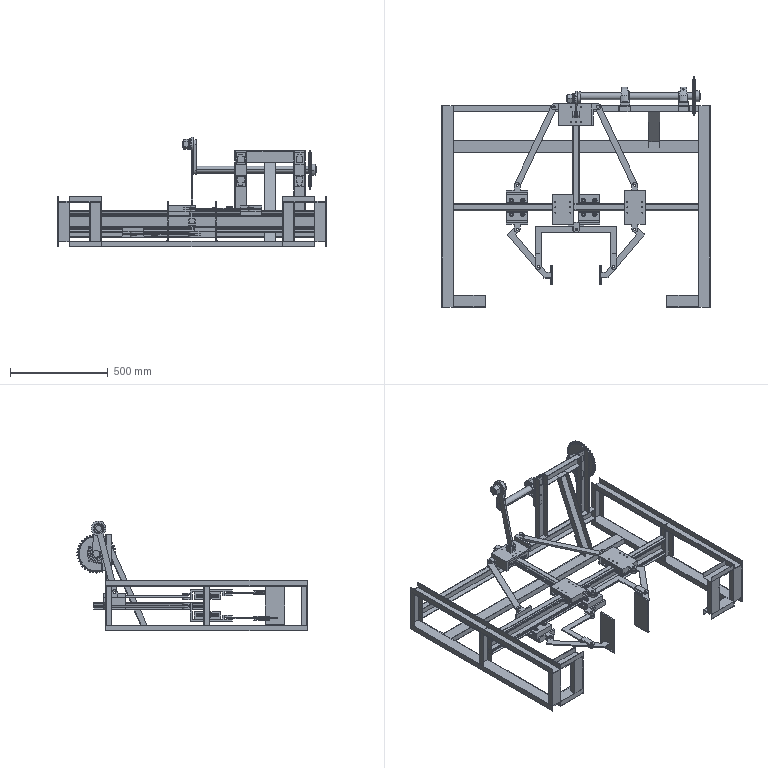Part | SolidWorks | features LocalLPattern 2, ReferencePattern 2 | 143 solids | 8967 faces | volume 12242540 mm3 | sphere 3008 | plane 2095 | cylinder 1821 | torus 1673 | cone 364 | spline 6 | commonest cylinder face diameters 22 x200 10 x172 13.5 x160 18.5 x160 11 x146 5 x120